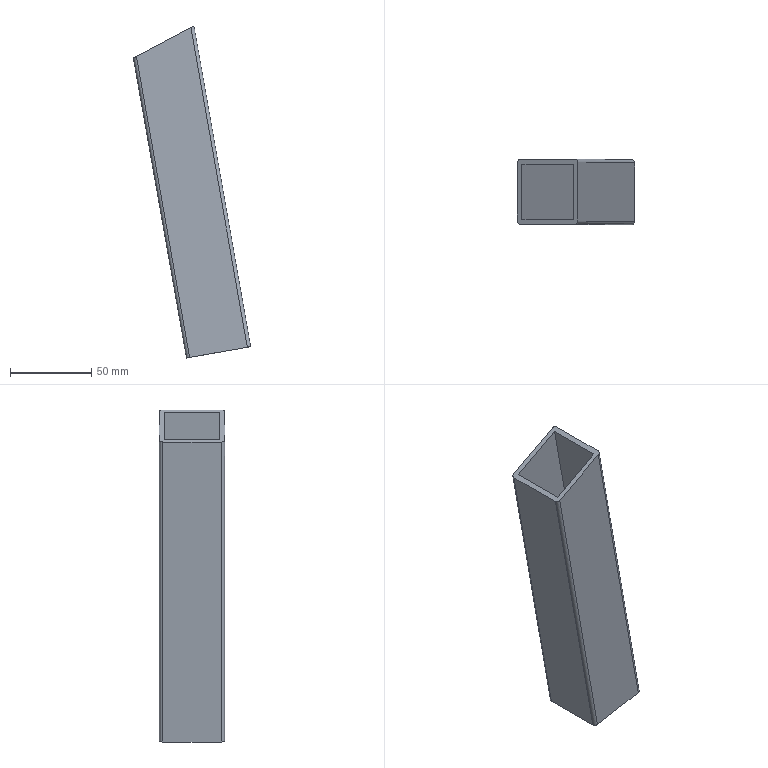Part | STEP file | diagonal bracket | 1 solid | 14 faces | box 71.941 x 40 x 203.909 mm | volume 85272 mm3 | plane 10 | cylinder 4 | commonest cylinder face diameters 4 x4
STEP:
#1=CARTESIAN_POINT('',(0.,0.,0.));
#2=DIRECTION('',(0.,0.,1.));
#3=DIRECTION('',(1.,0.,0.));
#4=AXIS2_PLACEMENT_3D('',#1,#2,#3);
#5=CARTESIAN_POINT('',(2102.233,153.75,-520.681));
#6=VERTEX_POINT('',#5);
#7=CARTESIAN_POINT('',(2068.752,153.75,-526.596));
#8=VERTEX_POINT('',#7);
#9=CARTESIAN_POINT('',(152.832,153.75,-865.079));
#10=DIRECTION('',(-0.9848,0.,-0.174));
#11=VECTOR('',#10,1.);
#12=LINE('',#9,#11);
#13=CARTESIAN_POINT('',(0.,153.75,0.));
#14=DIRECTION('',(0.,-1.,0.));
#15=DIRECTION('',(0.,0.,1.));
#16=AXIS2_PLACEMENT_3D('',#13,#14,#15);
#17=PLANE('',#16);
#18=CARTESIAN_POINT('',(-865.079,-152.832));
#19=DIRECTION('',(-0.174,0.9848));
#20=VECTOR('',#19,1.);
#21=LINE('',#18,#20);
#22=(GEOMETRIC_REPRESENTATION_CONTEXT(2)PARAMETRIC_REPRESENTATION_CONTEXT()REPRESENTATION_CONTEXT('',''));
#23=DEFINITIONAL_REPRESENTATION('',(#21),#22);
#24=PCURVE('',#17,#23);
#25=CARTESIAN_POINT('',(2105.187,190.75,-520.159));
#26=DIRECTION('',(-0.174,0.,0.9848));
#27=DIRECTION('',(-0.9848,0.,-0.174));
#28=AXIS2_PLACEMENT_3D('',#25,#26,#27);
#29=PLANE('',#28);
#30=CARTESIAN_POINT('',(1982.589,37.));
#31=DIRECTION('',(1.,0.));
#32=VECTOR('',#31,1.);
#33=LINE('',#30,#32);
#34=(GEOMETRIC_REPRESENTATION_CONTEXT(2)PARAMETRIC_REPRESENTATION_CONTEXT()REPRESENTATION_CONTEXT('',''));
#35=DEFINITIONAL_REPRESENTATION('',(#33),#34);
#36=PCURVE('',#29,#35);
#37=SURFACE_CURVE('',#12,(#24,#36),.PCURVE_S1.);
#38=EDGE_CURVE('',#6,#8,#37,.T.);
#39=ORIENTED_EDGE('',*,*,#38,.T.);
#40=CARTESIAN_POINT('',(2036.032,153.75,-341.393));
#41=VERTEX_POINT('',#40);
#42=CARTESIAN_POINT('',(2068.752,153.75,-526.596));
#43=DIRECTION('',(0.174,0.,-0.9848));
#44=VECTOR('',#43,1.);
#45=LINE('',#42,#44);
#46=CARTESIAN_POINT('',(-526.596,-2068.752));
#47=DIRECTION('',(-0.9848,-0.174));
#48=VECTOR('',#47,1.);
#49=LINE('',#46,#48);
#50=(GEOMETRIC_REPRESENTATION_CONTEXT(2)PARAMETRIC_REPRESENTATION_CONTEXT()REPRESENTATION_CONTEXT('',''));
#51=DEFINITIONAL_REPRESENTATION('',(#49),#50);
#52=PCURVE('',#17,#51);
#53=CARTESIAN_POINT('',(2068.752,190.75,-526.596));
#54=DIRECTION('',(0.9848,0.,0.174));
#55=DIRECTION('',(-0.174,0.,0.9848));
#56=AXIS2_PLACEMENT_3D('',#53,#54,#55);
#57=PLANE('',#56);
#58=CARTESIAN_POINT('',(0.,37.));
#59=DIRECTION('',(-1.,0.));
#60=VECTOR('',#59,1.);
#61=LINE('',#58,#60);
#62=(GEOMETRIC_REPRESENTATION_CONTEXT(2)PARAMETRIC_REPRESENTATION_CONTEXT()REPRESENTATION_CONTEXT('',''));
#63=DEFINITIONAL_REPRESENTATION('',(#61),#62);
#64=PCURVE('',#57,#63);
#65=SURFACE_CURVE('',#45,(#52,#64),.PCURVE_S1.);
#66=EDGE_CURVE('',#41,#8,#65,.T.);
#67=ORIENTED_EDGE('',*,*,#66,.F.);
#68=CARTESIAN_POINT('',(2067.606,153.75,-324.683));
#69=VERTEX_POINT('',#68);
#70=CARTESIAN_POINT('',(586.635,153.75,-1108.462));
#71=DIRECTION('',(0.8839,0.,0.4678));
#72=VECTOR('',#71,1.);
#73=LINE('',#70,#72);
#74=CARTESIAN_POINT('',(-1108.462,-586.635));
#75=DIRECTION('',(0.4678,-0.8839));
#76=VECTOR('',#75,1.);
#77=LINE('',#74,#76);
#78=(GEOMETRIC_REPRESENTATION_CONTEXT(2)PARAMETRIC_REPRESENTATION_CONTEXT()REPRESENTATION_CONTEXT('',''));
#79=DEFINITIONAL_REPRESENTATION('',(#77),#78);
#80=PCURVE('',#17,#79);
#81=CARTESIAN_POINT('',(2033.246,190.75,-342.868));
#82=DIRECTION('',(0.4678,0.,-0.8839));
#83=DIRECTION('',(0.8839,0.,0.4678));
#84=AXIS2_PLACEMENT_3D('',#81,#82,#83);
#85=PLANE('',#84);
#86=CARTESIAN_POINT('',(-1636.71,37.));
#87=DIRECTION('',(1.,0.));
#88=VECTOR('',#87,1.);
#89=LINE('',#86,#88);
#90=(GEOMETRIC_REPRESENTATION_CONTEXT(2)PARAMETRIC_REPRESENTATION_CONTEXT()REPRESENTATION_CONTEXT('',''));
#91=DEFINITIONAL_REPRESENTATION('',(#89),#90);
#92=PCURVE('',#85,#91);
#93=SURFACE_CURVE('',#73,(#80,#92),.PCURVE_S1.);
#94=EDGE_CURVE('',#41,#69,#93,.T.);
#95=ORIENTED_EDGE('',*,*,#94,.T.);
#96=CARTESIAN_POINT('',(2067.438,153.75,-323.73));
#97=DIRECTION('',(-0.174,0.,0.9848));
#98=VECTOR('',#97,1.);
#99=LINE('',#96,#98);
#100=CARTESIAN_POINT('',(-323.73,-2067.438));
#101=DIRECTION('',(0.9848,0.174));
#102=VECTOR('',#101,1.);
#103=LINE('',#100,#102);
#104=(GEOMETRIC_REPRESENTATION_CONTEXT(2)PARAMETRIC_REPRESENTATION_CONTEXT()REPRESENTATION_CONTEXT('',''));
#105=DEFINITIONAL_REPRESENTATION('',(#103),#104);
#106=PCURVE('',#17,#105);
#107=CARTESIAN_POINT('',(2067.438,190.75,-323.73));
#108=DIRECTION('',(-0.9848,0.,-0.174));
#109=DIRECTION('',(0.174,0.,-0.9848));
#110=AXIS2_PLACEMENT_3D('',#107,#108,#109);
#111=PLANE('',#110);
#112=CARTESIAN_POINT('',(0.,37.));
#113=DIRECTION('',(-1.,0.));
#114=VECTOR('',#113,1.);
#115=LINE('',#112,#114);
#116=(GEOMETRIC_REPRESENTATION_CONTEXT(2)PARAMETRIC_REPRESENTATION_CONTEXT()REPRESENTATION_CONTEXT('',''));
#117=DEFINITIONAL_REPRESENTATION('',(#115),#116);
#118=PCURVE('',#111,#117);
#119=SURFACE_CURVE('',#99,(#106,#118),.PCURVE_S1.);
#120=EDGE_CURVE('',#6,#69,#119,.T.);
#121=ORIENTED_EDGE('',*,*,#120,.F.);
#122=EDGE_LOOP('',(#39,#67,#95,#121));
#123=FACE_BOUND('',#122,.T.);
#124=ADVANCED_FACE('',(#123),#17,.F.);
#125=CARTESIAN_POINT('',(2036.032,187.75,-341.393));
#126=VERTEX_POINT('',#125);
#127=CARTESIAN_POINT('',(2067.606,187.75,-324.683));
#128=VERTEX_POINT('',#127);
#129=CARTESIAN_POINT('',(586.635,187.75,-1108.462));
#130=DIRECTION('',(0.8839,0.,0.4678));
#131=VECTOR('',#130,1.);
#132=LINE('',#129,#131);
#133=CARTESIAN_POINT('',(0.,187.75,0.));
#134=DIRECTION('',(0.,-1.,0.));
#135=DIRECTION('',(0.,0.,1.));
#136=AXIS2_PLACEMENT_3D('',#133,#134,#135);
#137=PLANE('',#136);
#138=CARTESIAN_POINT('',(-1108.462,-586.635));
#139=DIRECTION('',(0.4678,-0.8839));
#140=VECTOR('',#139,1.);
#141=LINE('',#138,#140);
#142=(GEOMETRIC_REPRESENTATION_CONTEXT(2)PARAMETRIC_REPRESENTATION_CONTEXT()REPRESENTATION_CONTEXT('',''));
#143=DEFINITIONAL_REPRESENTATION('',(#141),#142);
#144=PCURVE('',#137,#143);
#145=CARTESIAN_POINT('',(-1636.71,3.));
#146=DIRECTION('',(1.,0.));
#147=VECTOR('',#146,1.);
#148=LINE('',#145,#147);
#149=(GEOMETRIC_REPRESENTATION_CONTEXT(2)PARAMETRIC_REPRESENTATION_CONTEXT()REPRESENTATION_CONTEXT('',''));
#150=DEFINITIONAL_REPRESENTATION('',(#148),#149);
#151=PCURVE('',#85,#150);
#152=SURFACE_CURVE('',#132,(#144,#151),.PCURVE_S1.);
#153=EDGE_CURVE('',#126,#128,#152,.T.);
#154=ORIENTED_EDGE('',*,*,#153,.F.);
#155=CARTESIAN_POINT('',(2068.752,187.75,-526.596));
#156=VERTEX_POINT('',#155);
#157=CARTESIAN_POINT('',(2068.752,187.75,-526.596));
#158=DIRECTION('',(0.174,0.,-0.9848));
#159=VECTOR('',#158,1.);
#160=LINE('',#157,#159);
#161=CARTESIAN_POINT('',(-526.596,-2068.752));
#162=DIRECTION('',(-0.9848,-0.174));
#163=VECTOR('',#162,1.);
#164=LINE('',#161,#163);
#165=(GEOMETRIC_REPRESENTATION_CONTEXT(2)PARAMETRIC_REPRESENTATION_CONTEXT()REPRESENTATION_CONTEXT('',''));
#166=DEFINITIONAL_REPRESENTATION('',(#164),#165);
#167=PCURVE('',#137,#166);
#168=CARTESIAN_POINT('',(0.,3.));
#169=DIRECTION('',(-1.,0.));
#170=VECTOR('',#169,1.);
#171=LINE('',#168,#170);
#172=(GEOMETRIC_REPRESENTATION_CONTEXT(2)PARAMETRIC_REPRESENTATION_CONTEXT()REPRESENTATION_CONTEXT('',''));
#173=DEFINITIONAL_REPRESENTATION('',(#171),#172);
#174=PCURVE('',#57,#173);
#175=SURFACE_CURVE('',#160,(#167,#174),.PCURVE_S1.);
#176=EDGE_CURVE('',#126,#156,#175,.T.);
#177=ORIENTED_EDGE('',*,*,#176,.T.);
#178=CARTESIAN_POINT('',(2102.233,187.75,-520.681));
#179=VERTEX_POINT('',#178);
#180=CARTESIAN_POINT('',(152.832,187.75,-865.079));
#181=DIRECTION('',(-0.9848,0.,-0.174));
#182=VECTOR('',#181,1.);
#183=LINE('',#180,#182);
#184=CARTESIAN_POINT('',(-865.079,-152.832));
#185=DIRECTION('',(-0.174,0.9848));
#186=VECTOR('',#185,1.);
#187=LINE('',#184,#186);
#188=(GEOMETRIC_REPRESENTATION_CONTEXT(2)PARAMETRIC_REPRESENTATION_CONTEXT()REPRESENTATION_CONTEXT('',''));
#189=DEFINITIONAL_REPRESENTATION('',(#187),#188);
#190=PCURVE('',#137,#189);
#191=CARTESIAN_POINT('',(1982.589,3.));
#192=DIRECTION('',(1.,0.));
#193=VECTOR('',#192,1.);
#194=LINE('',#191,#193);
#195=(GEOMETRIC_REPRESENTATION_CONTEXT(2)PARAMETRIC_REPRESENTATION_CONTEXT()REPRESENTATION_CONTEXT('',''));
#196=DEFINITIONAL_REPRESENTATION('',(#194),#195);
#197=PCURVE('',#29,#196);
#198=SURFACE_CURVE('',#183,(#190,#197),.PCURVE_S1.);
#199=EDGE_CURVE('',#179,#156,#198,.T.);
#200=ORIENTED_EDGE('',*,*,#199,.F.);
#201=CARTESIAN_POINT('',(2067.438,187.75,-323.73));
#202=DIRECTION('',(-0.174,0.,0.9848));
#203=VECTOR('',#202,1.);
#204=LINE('',#201,#203);
#205=CARTESIAN_POINT('',(-323.73,-2067.438));
#206=DIRECTION('',(0.9848,0.174));
#207=VECTOR('',#206,1.);
#208=LINE('',#205,#207);
#209=(GEOMETRIC_REPRESENTATION_CONTEXT(2)PARAMETRIC_REPRESENTATION_CONTEXT()REPRESENTATION_CONTEXT('',''));
#210=DEFINITIONAL_REPRESENTATION('',(#208),#209);
#211=PCURVE('',#137,#210);
#212=CARTESIAN_POINT('',(0.,3.));
#213=DIRECTION('',(-1.,0.));
#214=VECTOR('',#213,1.);
#215=LINE('',#212,#214);
#216=(GEOMETRIC_REPRESENTATION_CONTEXT(2)PARAMETRIC_REPRESENTATION_CONTEXT()REPRESENTATION_CONTEXT('',''));
#217=DEFINITIONAL_REPRESENTATION('',(#215),#216);
#218=PCURVE('',#111,#217);
#219=SURFACE_CURVE('',#204,(#211,#218),.PCURVE_S1.);
#220=EDGE_CURVE('',#179,#128,#219,.T.);
#221=ORIENTED_EDGE('',*,*,#220,.T.);
#222=EDGE_LOOP('',(#154,#177,#200,#221));
#223=FACE_BOUND('',#222,.T.);
#224=ADVANCED_FACE('',(#223),#137,.T.);
#225=CARTESIAN_POINT('',(2067.606,190.75,-324.683));
#226=DIRECTION('',(0.,-1.,0.));
#227=VECTOR('',#226,1.);
#228=LINE('',#225,#227);
#229=CARTESIAN_POINT('',(0.9673,0.));
#230=DIRECTION('',(0.,1.));
#231=VECTOR('',#230,1.);
#232=LINE('',#229,#231);
#233=(GEOMETRIC_REPRESENTATION_CONTEXT(2)PARAMETRIC_REPRESENTATION_CONTEXT()REPRESENTATION_CONTEXT('',''));
#234=DEFINITIONAL_REPRESENTATION('',(#232),#233);
#235=PCURVE('',#111,#234);
#236=CARTESIAN_POINT('',(38.876,0.));
#237=DIRECTION('',(0.,1.));
#238=VECTOR('',#237,1.);
#239=LINE('',#236,#238);
#240=(GEOMETRIC_REPRESENTATION_CONTEXT(2)PARAMETRIC_REPRESENTATION_CONTEXT()REPRESENTATION_CONTEXT('',''));
#241=DEFINITIONAL_REPRESENTATION('',(#239),#240);
#242=PCURVE('',#85,#241);
#243=SURFACE_CURVE('',#228,(#235,#242),.PCURVE_S1.);
#244=EDGE_CURVE('',#128,#69,#243,.T.);
#245=ORIENTED_EDGE('',*,*,#244,.F.);
#246=ORIENTED_EDGE('',*,*,#220,.F.);
#247=CARTESIAN_POINT('',(2102.233,190.75,-520.681));
#248=DIRECTION('',(0.,-1.,0.));
#249=VECTOR('',#248,1.);
#250=LINE('',#247,#249);
#251=CARTESIAN_POINT('',(200.,0.));
#252=DIRECTION('',(0.,1.));
#253=VECTOR('',#252,1.);
#254=LINE('',#251,#253);
#255=(GEOMETRIC_REPRESENTATION_CONTEXT(2)PARAMETRIC_REPRESENTATION_CONTEXT()REPRESENTATION_CONTEXT('',''));
#256=DEFINITIONAL_REPRESENTATION('',(#254),#255);
#257=PCURVE('',#111,#256);
#258=CARTESIAN_POINT('',(3.,0.));
#259=DIRECTION('',(0.,1.));
#260=VECTOR('',#259,1.);
#261=LINE('',#258,#260);
#262=(GEOMETRIC_REPRESENTATION_CONTEXT(2)PARAMETRIC_REPRESENTATION_CONTEXT()REPRESENTATION_CONTEXT('',''));
#263=DEFINITIONAL_REPRESENTATION('',(#261),#262);
#264=PCURVE('',#29,#263);
#265=SURFACE_CURVE('',#250,(#257,#264),.PCURVE_S1.);
#266=EDGE_CURVE('',#179,#6,#265,.T.);
#267=ORIENTED_EDGE('',*,*,#266,.T.);
#268=ORIENTED_EDGE('',*,*,#120,.T.);
#269=EDGE_LOOP('',(#245,#246,#267,#268));
#270=FACE_BOUND('',#269,.T.);
#271=ADVANCED_FACE('',(#270),#111,.T.);
#272=CARTESIAN_POINT('',(2068.752,190.75,-526.596));
#273=DIRECTION('',(0.,-1.,0.));
#274=VECTOR('',#273,1.);
#275=LINE('',#272,#274);
#276=CARTESIAN_POINT('',(0.,0.));
#277=DIRECTION('',(0.,1.));
#278=VECTOR('',#277,1.);
#279=LINE('',#276,#278);
#280=(GEOMETRIC_REPRESENTATION_CONTEXT(2)PARAMETRIC_REPRESENTATION_CONTEXT()REPRESENTATION_CONTEXT('',''));
#281=DEFINITIONAL_REPRESENTATION('',(#279),#280);
#282=PCURVE('',#57,#281);
#283=CARTESIAN_POINT('',(37.,0.));
#284=DIRECTION('',(0.,1.));
#285=VECTOR('',#284,1.);
#286=LINE('',#283,#285);
#287=(GEOMETRIC_REPRESENTATION_CONTEXT(2)PARAMETRIC_REPRESENTATION_CONTEXT()REPRESENTATION_CONTEXT('',''));
#288=DEFINITIONAL_REPRESENTATION('',(#286),#287);
#289=PCURVE('',#29,#288);
#290=SURFACE_CURVE('',#275,(#282,#289),.PCURVE_S1.);
#291=EDGE_CURVE('',#156,#8,#290,.T.);
#292=ORIENTED_EDGE('',*,*,#291,.F.);
#293=ORIENTED_EDGE('',*,*,#176,.F.);
#294=CARTESIAN_POINT('',(2036.032,190.75,-341.393));
#295=DIRECTION('',(0.,-1.,0.));
#296=VECTOR('',#295,1.);
#297=LINE('',#294,#296);
#298=CARTESIAN_POINT('',(188.071,0.));
#299=DIRECTION('',(0.,1.));
#300=VECTOR('',#299,1.);
#301=LINE('',#298,#300);
#302=(GEOMETRIC_REPRESENTATION_CONTEXT(2)PARAMETRIC_REPRESENTATION_CONTEXT()REPRESENTATION_CONTEXT('',''));
#303=DEFINITIONAL_REPRESENTATION('',(#301),#302);
#304=PCURVE('',#57,#303);
#305=CARTESIAN_POINT('',(3.152,0.));
#306=DIRECTION('',(0.,1.));
#307=VECTOR('',#306,1.);
#308=LINE('',#305,#307);
#309=(GEOMETRIC_REPRESENTATION_CONTEXT(2)PARAMETRIC_REPRESENTATION_CONTEXT()REPRESENTATION_CONTEXT('',''));
#310=DEFINITIONAL_REPRESENTATION('',(#308),#309);
#311=PCURVE('',#85,#310);
#312=SURFACE_CURVE('',#297,(#304,#311),.PCURVE_S1.);
#313=EDGE_CURVE('',#126,#41,#312,.T.);
#314=ORIENTED_EDGE('',*,*,#313,.T.);
#315=ORIENTED_EDGE('',*,*,#66,.T.);
#316=EDGE_LOOP('',(#292,#293,#314,#315));
#317=FACE_BOUND('',#316,.T.);
#318=ADVANCED_FACE('',(#317),#57,.T.);
#319=CARTESIAN_POINT('',(2065.797,188.75,-527.118));
#320=VERTEX_POINT('',#319);
#321=CARTESIAN_POINT('',(2067.767,190.75,-526.77));
#322=VERTEX_POINT('',#321);
#323=CARTESIAN_POINT('',(2067.767,188.75,-526.77));
#324=DIRECTION('',(0.174,0.,-0.9848));
#325=DIRECTION('',(0.9848,0.,0.174));
#326=AXIS2_PLACEMENT_3D('',#323,#324,#325);
#327=CIRCLE('',#326,2.);
#328=CARTESIAN_POINT('',(1914.935,188.75,338.309));
#329=DIRECTION('',(-0.174,0.,0.9848));
#330=DIRECTION('',(-0.9848,0.,-0.174));
#331=AXIS2_PLACEMENT_3D('',#328,#329,#330);
#332=CYLINDRICAL_SURFACE('',#331,2.);
#333=CARTESIAN_POINT('',(9.425,-878.475));
#334=DIRECTION('',(-1.,0.));
#335=VECTOR('',#334,1.);
#336=LINE('',#333,#335);
#337=(GEOMETRIC_REPRESENTATION_CONTEXT(2)PARAMETRIC_REPRESENTATION_CONTEXT()REPRESENTATION_CONTEXT('',''));
#338=DEFINITIONAL_REPRESENTATION('',(#336),#337);
#339=PCURVE('',#332,#338);
#340=CARTESIAN_POINT('',(36.,2.));
#341=CARTESIAN_POINT('',(36.,5.464));
#342=CARTESIAN_POINT('',(39.,3.732));
#343=CARTESIAN_POINT('',(42.,2.));
#344=CARTESIAN_POINT('',(39.,0.2679));
#345=CARTESIAN_POINT('',(36.,-1.464));
#346=CARTESIAN_POINT('',(36.,2.));
#347=(BOUNDED_CURVE()B_SPLINE_CURVE(2,(#340,#341,#342,#343,#344,#345,#346),.UNSPECIFIED.,.T.,.F.)B_SPLINE_CURVE_WITH_KNOTS((1,2,2,2,2,1),(-2.094,0.,2.094,4.189,6.283,8.378),.UNSPECIFIED.)CURVE()GEOMETRIC_REPRESENTATION_ITEM()RATIONAL_B_SPLINE_CURVE((1.,0.5,1.,0.5,1.,0.5,1.))REPRESENTATION_ITEM(''));
#348=(GEOMETRIC_REPRESENTATION_CONTEXT(2)PARAMETRIC_REPRESENTATION_CONTEXT()REPRESENTATION_CONTEXT('',''));
#349=DEFINITIONAL_REPRESENTATION('',(#347),#348);
#350=PCURVE('',#29,#349);
#351=SURFACE_CURVE('',#327,(#339,#350),.PCURVE_S1.);
#352=EDGE_CURVE('',#320,#322,#351,.T.);
#353=ORIENTED_EDGE('',*,*,#352,.F.);
#354=CARTESIAN_POINT('',(2033.246,188.75,-342.868));
#355=VERTEX_POINT('',#354);
#356=CARTESIAN_POINT('',(2065.797,188.75,-527.118));
#357=DIRECTION('',(0.174,0.,-0.9848));
#358=VECTOR('',#357,1.);
#359=LINE('',#356,#358);
#360=CARTESIAN_POINT('',(6.283,-878.475));
#361=DIRECTION('',(0.,-1.));
#362=VECTOR('',#361,1.);
#363=LINE('',#360,#362);
#364=(GEOMETRIC_REPRESENTATION_CONTEXT(2)PARAMETRIC_REPRESENTATION_CONTEXT()REPRESENTATION_CONTEXT('',''));
#365=DEFINITIONAL_REPRESENTATION('',(#363),#364);
#366=PCURVE('',#332,#365);
#367=CARTESIAN_POINT('',(2065.797,190.75,-527.118));
#368=DIRECTION('',(0.9848,0.,0.174));
#369=DIRECTION('',(-0.174,0.,0.9848));
#370=AXIS2_PLACEMENT_3D('',#367,#368,#369);
#371=PLANE('',#370);
#372=CARTESIAN_POINT('',(0.,2.));
#373=DIRECTION('',(-1.,0.));
#374=VECTOR('',#373,1.);
#375=LINE('',#372,#374);
#376=(GEOMETRIC_REPRESENTATION_CONTEXT(2)PARAMETRIC_REPRESENTATION_CONTEXT()REPRESENTATION_CONTEXT('',''));
#377=DEFINITIONAL_REPRESENTATION('',(#375),#376);
#378=PCURVE('',#371,#377);
#379=SURFACE_CURVE('',#359,(#366,#378),.PCURVE_S1.);
#380=EDGE_CURVE('',#355,#320,#379,.T.);
#381=ORIENTED_EDGE('',*,*,#380,.F.);
#382=CARTESIAN_POINT('',(2035.103,190.75,-341.885));
#383=VERTEX_POINT('',#382);
#384=CARTESIAN_POINT('',(2035.103,188.75,-341.885));
#385=DIRECTION('',(-0.4678,0.,0.8839));
#386=DIRECTION('',(0.8839,0.,0.4678));
#387=AXIS2_PLACEMENT_3D('',#384,#385,#386);
#388=ELLIPSE('',#387,2.101,2.);
#389=CARTESIAN_POINT('',(4.712,-690.727));
#390=CARTESIAN_POINT('',(4.736,-690.742));
#391=CARTESIAN_POINT('',(4.784,-690.773));
#392=CARTESIAN_POINT('',(4.855,-690.819));
#393=CARTESIAN_POINT('',(4.927,-690.864));
#394=CARTESIAN_POINT('',(4.998,-690.909));
#395=CARTESIAN_POINT('',(5.069,-690.953));
#396=CARTESIAN_POINT('',(5.141,-690.995));
#397=CARTESIAN_POINT('',(5.212,-691.036));
#398=CARTESIAN_POINT('',(5.284,-691.076));
#399=CARTESIAN_POINT('',(5.355,-691.114));
#400=CARTESIAN_POINT('',(5.426,-691.15));
#401=CARTESIAN_POINT('',(5.498,-691.183));
#402=CARTESIAN_POINT('',(5.569,-691.215));
#403=CARTESIAN_POINT('',(5.641,-691.244));
#404=CARTESIAN_POINT('',(5.712,-691.27));
#405=CARTESIAN_POINT('',(5.783,-691.294));
#406=CARTESIAN_POINT('',(5.855,-691.314));
#407=CARTESIAN_POINT('',(5.926,-691.332));
#408=CARTESIAN_POINT('',(5.998,-691.346));
#409=CARTESIAN_POINT('',(6.069,-691.358));
#410=CARTESIAN_POINT('',(6.14,-691.366));
#411=CARTESIAN_POINT('',(6.212,-691.371));
#412=CARTESIAN_POINT('',(6.259,-691.372));
#413=CARTESIAN_POINT('',(6.283,-691.372));
#414=B_SPLINE_CURVE_WITH_KNOTS('',3,(#389,#390,#391,#392,#393,#394,#395,#396,#397,#398,#399,#400,#401,#402,#403,#404,#405,#406,#407,#408,#409,#410,#411,#412,#413),.UNSPECIFIED.,.F.,.F.,(4,1,1,1,1,1,1,1,1,1,1,1,1,1,1,1,1,1,1,1,1,1,4),(1.571,1.642,1.714,1.785,1.856,1.928,1.999,2.071,2.142,2.213,2.285,2.356,2.428,2.499,2.57,2.642,2.713,2.785,2.856,2.927,2.999,3.07,3.142),.QUASI_UNIFORM_KNOTS.);
#415=(GEOMETRIC_REPRESENTATION_CONTEXT(2)PARAMETRIC_REPRESENTATION_CONTEXT()REPRESENTATION_CONTEXT('',''));
#416=DEFINITIONAL_REPRESENTATION('',(#414),#415);
#417=PCURVE('',#332,#416);
#418=CARTESIAN_POINT('',(4.203,2.));
#419=CARTESIAN_POINT('',(4.203,-1.464));
#420=CARTESIAN_POINT('',(1.051,0.2679));
#421=CARTESIAN_POINT('',(-2.101,2.));
#422=CARTESIAN_POINT('',(1.051,3.732));
#423=CARTESIAN_POINT('',(4.203,5.464));
#424=CARTESIAN_POINT('',(4.203,2.));
#425=(BOUNDED_CURVE()B_SPLINE_CURVE(2,(#418,#419,#420,#421,#422,#423,#424),.UNSPECIFIED.,.T.,.F.)B_SPLINE_CURVE_WITH_KNOTS((1,2,2,2,2,1),(-2.094,0.,2.094,4.189,6.283,8.378),.UNSPECIFIED.)CURVE()GEOMETRIC_REPRESENTATION_ITEM()RATIONAL_B_SPLINE_CURVE((1.,0.5,1.,0.5,1.,0.5,1.))REPRESENTATION_ITEM(''));
#426=(GEOMETRIC_REPRESENTATION_CONTEXT(2)PARAMETRIC_REPRESENTATION_CONTEXT()REPRESENTATION_CONTEXT('',''));
#427=DEFINITIONAL_REPRESENTATION('',(#425),#426);
#428=PCURVE('',#85,#427);
#429=SURFACE_CURVE('',#388,(#417,#428),.PCURVE_S1.);
#430=EDGE_CURVE('',#383,#355,#429,.T.);
#431=ORIENTED_EDGE('',*,*,#430,.F.);
#432=CARTESIAN_POINT('',(1914.935,190.75,338.309));
#433=DIRECTION('',(-0.174,0.,0.9848));
#434=VECTOR('',#433,1.);
#435=LINE('',#432,#434);
#436=CARTESIAN_POINT('',(4.712,0.));
#437=DIRECTION('',(0.,1.));
#438=VECTOR('',#437,1.);
#439=LINE('',#436,#438);
#440=(GEOMETRIC_REPRESENTATION_CONTEXT(2)PARAMETRIC_REPRESENTATION_CONTEXT()REPRESENTATION_CONTEXT('',''));
#441=DEFINITIONAL_REPRESENTATION('',(#439),#440);
#442=PCURVE('',#332,#441);
#443=CARTESIAN_POINT('',(0.,190.75,0.));
#444=DIRECTION('',(0.,-1.,0.));
#445=DIRECTION('',(0.,0.,1.));
#446=AXIS2_PLACEMENT_3D('',#443,#444,#445);
#447=PLANE('',#446);
#448=CARTESIAN_POINT('',(338.309,-1914.935));
#449=DIRECTION('',(0.9848,0.174));
#450=VECTOR('',#449,1.);
#451=LINE('',#448,#450);
#452=(GEOMETRIC_REPRESENTATION_CONTEXT(2)PARAMETRIC_REPRESENTATION_CONTEXT()REPRESENTATION_CONTEXT('',''));
#453=DEFINITIONAL_REPRESENTATION('',(#451),#452);
#454=PCURVE('',#447,#453);
#455=SURFACE_CURVE('',#435,(#442,#454),.PCURVE_S1.);
#456=EDGE_CURVE('',#322,#383,#455,.T.);
#457=ORIENTED_EDGE('',*,*,#456,.F.);
#458=EDGE_LOOP('',(#353,#381,#431,#457));
#459=FACE_BOUND('',#458,.T.);
#460=ADVANCED_FACE('',(#459),#332,.T.);
#461=CARTESIAN_POINT('',(2070.392,188.75,-323.209));
#462=VERTEX_POINT('',#461);
#463=CARTESIAN_POINT('',(2068.535,190.75,-324.192));
#464=VERTEX_POINT('',#463);
#465=CARTESIAN_POINT('',(2068.535,188.75,-324.192));
#466=DIRECTION('',(-0.4678,0.,0.8839));
#467=DIRECTION('',(-0.8839,0.,-0.4678));
#468=AXIS2_PLACEMENT_3D('',#465,#466,#467);
#469=ELLIPSE('',#468,2.101,2.);
#470=CARTESIAN_POINT('',(1950.386,188.75,344.572));
#471=DIRECTION('',(0.174,0.,-0.9848));
#472=DIRECTION('',(0.9848,0.,0.174));
#473=AXIS2_PLACEMENT_3D('',#470,#471,#472);
#474=CYLINDRICAL_SURFACE('',#473,2.);
#475=CARTESIAN_POINT('',(6.283,678.475));
#476=CARTESIAN_POINT('',(6.259,678.475));
#477=CARTESIAN_POINT('',(6.212,678.476));
#478=CARTESIAN_POINT('',(6.14,678.481));
#479=CARTESIAN_POINT('',(6.069,678.489));
#480=CARTESIAN_POINT('',(5.998,678.501));
#481=CARTESIAN_POINT('',(5.926,678.515));
#482=CARTESIAN_POINT('',(5.855,678.533));
#483=CARTESIAN_POINT('',(5.783,678.554));
#484=CARTESIAN_POINT('',(5.712,678.577));
#485=CARTESIAN_POINT('',(5.641,678.603));
#486=CARTESIAN_POINT('',(5.569,678.632));
#487=CARTESIAN_POINT('',(5.498,678.664));
#488=CARTESIAN_POINT('',(5.426,678.697));
#489=CARTESIAN_POINT('',(5.355,678.733));
#490=CARTESIAN_POINT('',(5.284,678.771));
#491=CARTESIAN_POINT('',(5.212,678.811));
#492=CARTESIAN_POINT('',(5.141,678.852));
#493=CARTESIAN_POINT('',(5.069,678.895));
#494=CARTESIAN_POINT('',(4.998,678.938));
#495=CARTESIAN_POINT('',(4.927,678.983));
#496=CARTESIAN_POINT('',(4.855,679.028));
#497=CARTESIAN_POINT('',(4.784,679.074));
#498=CARTESIAN_POINT('',(4.736,679.105));
#499=CARTESIAN_POINT('',(4.712,679.12));
#500=B_SPLINE_CURVE_WITH_KNOTS('',3,(#475,#476,#477,#478,#479,#480,#481,#482,#483,#484,#485,#486,#487,#488,#489,#490,#491,#492,#493,#494,#495,#496,#497,#498,#499),.UNSPECIFIED.,.F.,.F.,(4,1,1,1,1,1,1,1,1,1,1,1,1,1,1,1,1,1,1,1,1,1,4),(3.142,3.213,3.284,3.356,3.427,3.499,3.57,3.641,3.713,3.784,3.856,3.927,3.998,4.07,4.141,4.213,4.284,4.355,4.427,4.498,4.57,4.641,4.712),.QUASI_UNIFORM_KNOTS.);
#501=(GEOMETRIC_REPRESENTATION_CONTEXT(2)PARAMETRIC_REPRESENTATION_CONTEXT()REPRESENTATION_CONTEXT('',''));
#502=DEFINITIONAL_REPRESENTATION('',(#500),#501);
#503=PCURVE('',#474,#502);
#504=CARTESIAN_POINT('',(37.825,2.));
#505=CARTESIAN_POINT('',(37.825,5.464));
#506=CARTESIAN_POINT('',(40.977,3.732));
#507=CARTESIAN_POINT('',(44.129,2.));
#508=CARTESIAN_POINT('',(40.977,0.2679));
#509=CARTESIAN_POINT('',(37.825,-1.464));
#510=CARTESIAN_POINT('',(37.825,2.));
#511=(BOUNDED_CURVE()B_SPLINE_CURVE(2,(#504,#505,#506,#507,#508,#509,#510),.UNSPECIFIED.,.T.,.F.)B_SPLINE_CURVE_WITH_KNOTS((1,2,2,2,2,1),(-2.094,0.,2.094,4.189,6.283,8.378),.UNSPECIFIED.)CURVE()GEOMETRIC_REPRESENTATION_ITEM()RATIONAL_B_SPLINE_CURVE((1.,0.5,1.,0.5,1.,0.5,1.))REPRESENTATION_ITEM(''));
#512=(GEOMETRIC_REPRESENTATION_CONTEXT(2)PARAMETRIC_REPRESENTATION_CONTEXT()REPRESENTATION_CONTEXT('',''));
#513=DEFINITIONAL_REPRESENTATION('',(#511),#512);
#514=PCURVE('',#85,#513);
#515=SURFACE_CURVE('',#469,(#503,#514),.PCURVE_S1.);
#516=EDGE_CURVE('',#462,#464,#515,.T.);
#517=ORIENTED_EDGE('',*,*,#516,.F.);
#518=CARTESIAN_POINT('',(2105.187,188.75,-520.159));
#519=VERTEX_POINT('',#518);
#520=CARTESIAN_POINT('',(2070.392,188.75,-323.209));
#521=DIRECTION('',(-0.174,0.,0.9848));
#522=VECTOR('',#521,1.);
#523=LINE('',#520,#522);
#524=CARTESIAN_POINT('',(6.283,678.475));
#525=DIRECTION('',(0.,-1.));
#526=VECTOR('',#525,1.);
#527=LINE('',#524,#526);
#528=(GEOMETRIC_REPRESENTATION_CONTEXT(2)PARAMETRIC_REPRESENTATION_CONTEXT()REPRESENTATION_CONTEXT('',''));
#529=DEFINITIONAL_REPRESENTATION('',(#527),#528);
#530=PCURVE('',#474,#529);
#531=CARTESIAN_POINT('',(2070.392,190.75,-323.209));
#532=DIRECTION('',(-0.9848,0.,-0.174));
#533=DIRECTION('',(0.174,0.,-0.9848));
#534=AXIS2_PLACEMENT_3D('',#531,#532,#533);
#535=PLANE('',#534);
#536=CARTESIAN_POINT('',(0.,2.));
#537=DIRECTION('',(-1.,0.));
#538=VECTOR('',#537,1.);
#539=LINE('',#536,#538);
#540=(GEOMETRIC_REPRESENTATION_CONTEXT(2)PARAMETRIC_REPRESENTATION_CONTEXT()REPRESENTATION_CONTEXT('',''));
#541=DEFINITIONAL_REPRESENTATION('',(#539),#540);
#542=PCURVE('',#535,#541);
#543=SURFACE_CURVE('',#523,(#530,#542),.PCURVE_S1.);
#544=EDGE_CURVE('',#519,#462,#543,.T.);
#545=ORIENTED_EDGE('',*,*,#544,.F.);
#546=CARTESIAN_POINT('',(2103.218,190.75,-520.507));
#547=VERTEX_POINT('',#546);
#548=CARTESIAN_POINT('',(2103.218,188.75,-520.507));
#549=DIRECTION('',(0.174,0.,-0.9848));
#550=DIRECTION('',(0.9848,0.,0.174));
#551=AXIS2_PLACEMENT_3D('',#548,#549,#550);
#552=CIRCLE('',#551,2.);
#553=CARTESIAN_POINT('',(0.,878.475));
#554=DIRECTION('',(1.,0.));
#555=VECTOR('',#554,1.);
#556=LINE('',#553,#555);
#557=(GEOMETRIC_REPRESENTATION_CONTEXT(2)PARAMETRIC_REPRESENTATION_CONTEXT()REPRESENTATION_CONTEXT('',''));
#558=DEFINITIONAL_REPRESENTATION('',(#556),#557);
#559=PCURVE('',#474,#558);
#560=CARTESIAN_POINT('',(0.,2.));
#561=CARTESIAN_POINT('',(0.,5.464));
#562=CARTESIAN_POINT('',(3.,3.732));
#563=CARTESIAN_POINT('',(6.,2.));
#564=CARTESIAN_POINT('',(3.,0.2679));
#565=CARTESIAN_POINT('',(0.,-1.464));
#566=CARTESIAN_POINT('',(0.,2.));
#567=(BOUNDED_CURVE()B_SPLINE_CURVE(2,(#560,#561,#562,#563,#564,#565,#566),.UNSPECIFIED.,.T.,.F.)B_SPLINE_CURVE_WITH_KNOTS((1,2,2,2,2,1),(-2.094,0.,2.094,4.189,6.283,8.378),.UNSPECIFIED.)CURVE()GEOMETRIC_REPRESENTATION_ITEM()RATIONAL_B_SPLINE_CURVE((1.,0.5,1.,0.5,1.,0.5,1.))REPRESENTATION_ITEM(''));
#568=(GEOMETRIC_REPRESENTATION_CONTEXT(2)PARAMETRIC_REPRESENTATION_CONTEXT()REPRESENTATION_CONTEXT('',''));
#569=DEFINITIONAL_REPRESENTATION('',(#567),#568);
#570=PCURVE('',#29,#569);
#571=SURFACE_CURVE('',#552,(#559,#570),.PCURVE_S1.);
#572=EDGE_CURVE('',#547,#519,#571,.T.);
#573=ORIENTED_EDGE('',*,*,#572,.F.);
#574=CARTESIAN_POINT('',(1950.386,190.75,344.572));
#575=DIRECTION('',(0.174,0.,-0.9848));
#576=VECTOR('',#575,1.);
#577=LINE('',#574,#576);
#578=CARTESIAN_POINT('',(4.712,0.));
#579=DIRECTION('',(0.,1.));
#580=VECTOR('',#579,1.);
#581=LINE('',#578,#580);
#582=(GEOMETRIC_REPRESENTATION_CONTEXT(2)PARAMETRIC_REPRESENTATION_CONTEXT()REPRESENTATION_CONTEXT('',''));
#583=DEFINITIONAL_REPRESENTATION('',(#581),#582);
#584=PCURVE('',#474,#583);
#585=CARTESIAN_POINT('',(344.572,-1950.386));
#586=DIRECTION('',(-0.9848,-0.174));
#587=VECTOR('',#586,1.);
#588=LINE('',#585,#587);
#589=(GEOMETRIC_REPRESENTATION_CONTEXT(2)PARAMETRIC_REPRESENTATION_CONTEXT()REPRESENTATION_CONTEXT('',''));
#590=DEFINITIONAL_REPRESENTATION('',(#588),#589);
#591=PCURVE('',#447,#590);
#592=SURFACE_CURVE('',#577,(#584,#591),.PCURVE_S1.);
#593=EDGE_CURVE('',#464,#547,#592,.T.);
#594=ORIENTED_EDGE('',*,*,#593,.F.);
#595=EDGE_LOOP('',(#517,#545,#573,#594));
#596=FACE_BOUND('',#595,.T.);
#597=ADVANCED_FACE('',(#596),#474,.T.);
#598=CARTESIAN_POINT('',(2067.767,150.75,-526.77));
#599=VERTEX_POINT('',#598);
#600=CARTESIAN_POINT('',(2065.797,152.75,-527.118));
#601=VERTEX_POINT('',#600);
#602=CARTESIAN_POINT('',(2067.767,152.75,-526.77));
#603=DIRECTION('',(0.174,0.,-0.9848));
#604=DIRECTION('',(0.9848,0.,0.174));
#605=AXIS2_PLACEMENT_3D('',#602,#603,#604);
#606=CIRCLE('',#605,2.);
#607=CARTESIAN_POINT('',(2067.767,152.75,-526.77));
#608=DIRECTION('',(0.174,0.,-0.9848));
#609=DIRECTION('',(0.9848,0.,0.174));
#610=AXIS2_PLACEMENT_3D('',#607,#608,#609);
#611=CYLINDRICAL_SURFACE('',#610,2.);
#612=CARTESIAN_POINT('',(0.,0.));
#613=DIRECTION('',(1.,0.));
#614=VECTOR('',#613,1.);
#615=LINE('',#612,#614);
#616=(GEOMETRIC_REPRESENTATION_CONTEXT(2)PARAMETRIC_REPRESENTATION_CONTEXT()REPRESENTATION_CONTEXT('',''));
#617=DEFINITIONAL_REPRESENTATION('',(#615),#616);
#618=PCURVE('',#611,#617);
#619=CARTESIAN_POINT('',(36.,38.));
#620=CARTESIAN_POINT('',(36.,41.464));
#621=CARTESIAN_POINT('',(39.,39.732));
#622=CARTESIAN_POINT('',(42.,38.));
#623=CARTESIAN_POINT('',(39.,36.268));
#624=CARTESIAN_POINT('',(36.,34.536));
#625=CARTESIAN_POINT('',(36.,38.));
#626=(BOUNDED_CURVE()B_SPLINE_CURVE(2,(#619,#620,#621,#622,#623,#624,#625),.UNSPECIFIED.,.T.,.F.)B_SPLINE_CURVE_WITH_KNOTS((1,2,2,2,2,1),(-2.094,0.,2.094,4.189,6.283,8.378),.UNSPECIFIED.)CURVE()GEOMETRIC_REPRESENTATION_ITEM()RATIONAL_B_SPLINE_CURVE((1.,0.5,1.,0.5,1.,0.5,1.))REPRESENTATION_ITEM(''));
#627=(GEOMETRIC_REPRESENTATION_CONTEXT(2)PARAMETRIC_REPRESENTATION_CONTEXT()REPRESENTATION_CONTEXT('',''));
#628=DEFINITIONAL_REPRESENTATION('',(#626),#627);
#629=PCURVE('',#29,#628);
#630=SURFACE_CURVE('',#606,(#618,#629),.PCURVE_S1.);
#631=EDGE_CURVE('',#599,#601,#630,.T.);
#632=ORIENTED_EDGE('',*,*,#631,.F.);
#633=CARTESIAN_POINT('',(2035.103,150.75,-341.885));
#634=VERTEX_POINT('',#633);
#635=CARTESIAN_POINT('',(2067.767,150.75,-526.77));
#636=DIRECTION('',(0.174,0.,-0.9848));
#637=VECTOR('',#636,1.);
#638=LINE('',#635,#637);
#639=CARTESIAN_POINT('',(1.571,0.));
#640=DIRECTION('',(0.,1.));
#641=VECTOR('',#640,1.);
#642=LINE('',#639,#641);
#643=(GEOMETRIC_REPRESENTATION_CONTEXT(2)PARAMETRIC_REPRESENTATION_CONTEXT()REPRESENTATION_CONTEXT('',''));
#644=DEFINITIONAL_REPRESENTATION('',(#642),#643);
#645=PCURVE('',#611,#644);
#646=CARTESIAN_POINT('',(0.,150.75,0.));
#647=DIRECTION('',(0.,-1.,0.));
#648=DIRECTION('',(0.,0.,1.));
#649=AXIS2_PLACEMENT_3D('',#646,#647,#648);
#650=PLANE('',#649);
#651=CARTESIAN_POINT('',(-526.77,-2067.767));
#652=DIRECTION('',(-0.9848,-0.174));
#653=VECTOR('',#652,1.);
#654=LINE('',#651,#653);
#655=(GEOMETRIC_REPRESENTATION_CONTEXT(2)PARAMETRIC_REPRESENTATION_CONTEXT()REPRESENTATION_CONTEXT('',''));
#656=DEFINITIONAL_REPRESENTATION('',(#654),#655);
#657=PCURVE('',#650,#656);
#658=SURFACE_CURVE('',#638,(#645,#657),.PCURVE_S1.);
#659=EDGE_CURVE('',#634,#599,#658,.T.);
#660=ORIENTED_EDGE('',*,*,#659,.F.);
#661=CARTESIAN_POINT('',(2033.246,152.75,-342.868));
#662=VERTEX_POINT('',#661);
#663=CARTESIAN_POINT('',(2035.103,152.75,-341.885));
#664=DIRECTION('',(-0.4678,0.,0.8839));
#665=DIRECTION('',(-0.8839,0.,-0.4678));
#666=AXIS2_PLACEMENT_3D('',#663,#664,#665);
#667=ELLIPSE('',#666,2.101,2.);
#668=CARTESIAN_POINT('',(3.142,-187.103));
#669=CARTESIAN_POINT('',(3.118,-187.103));
#670=CARTESIAN_POINT('',(3.07,-187.104));
#671=CARTESIAN_POINT('',(2.999,-187.109));
#672=CARTESIAN_POINT('',(2.927,-187.117));
#673=CARTESIAN_POINT('',(2.856,-187.129));
#674=CARTESIAN_POINT('',(2.785,-187.143));
#675=CARTESIAN_POINT('',(2.713,-187.161));
#676=CARTESIAN_POINT('',(2.642,-187.182));
#677=CARTESIAN_POINT('',(2.57,-187.205));
#678=CARTESIAN_POINT('',(2.499,-187.231));
#679=CARTESIAN_POINT('',(2.428,-187.26));
#680=CARTESIAN_POINT('',(2.356,-187.292));
#681=CARTESIAN_POINT('',(2.285,-187.325));
#682=CARTESIAN_POINT('',(2.213,-187.361));
#683=CARTESIAN_POINT('',(2.142,-187.399));
#684=CARTESIAN_POINT('',(2.071,-187.439));
#685=CARTESIAN_POINT('',(1.999,-187.48));
#686=CARTESIAN_POINT('',(1.928,-187.523));
#687=CARTESIAN_POINT('',(1.856,-187.566));
#688=CARTESIAN_POINT('',(1.785,-187.611));
#689=CARTESIAN_POINT('',(1.714,-187.656));
#690=CARTESIAN_POINT('',(1.642,-187.702));
#691=CARTESIAN_POINT('',(1.595,-187.733));
#692=CARTESIAN_POINT('',(1.571,-187.748));
#693=B_SPLINE_CURVE_WITH_KNOTS('',3,(#668,#669,#670,#671,#672,#673,#674,#675,#676,#677,#678,#679,#680,#681,#682,#683,#684,#685,#686,#687,#688,#689,#690,#691,#692),.UNSPECIFIED.,.F.,.F.,(4,1,1,1,1,1,1,1,1,1,1,1,1,1,1,1,1,1,1,1,1,1,4),(0.,0.0714,0.1428,0.2142,0.2856,0.357,0.4284,0.4998,0.5712,0.6426,0.714,0.7854,0.8568,0.9282,0.9996,1.071,1.142,1.214,1.285,1.357,1.428,1.499,1.571),.QUASI_UNIFORM_KNOTS.);
#694=(GEOMETRIC_REPRESENTATION_CONTEXT(2)PARAMETRIC_REPRESENTATION_CONTEXT()REPRESENTATION_CONTEXT('',''));
#695=DEFINITIONAL_REPRESENTATION('',(#693),#694);
#696=PCURVE('',#611,#695);
#697=CARTESIAN_POINT('',(0.,38.));
#698=CARTESIAN_POINT('',(0.,41.464));
#699=CARTESIAN_POINT('',(3.152,39.732));
#700=CARTESIAN_POINT('',(6.304,38.));
#701=CARTESIAN_POINT('',(3.152,36.268));
#702=CARTESIAN_POINT('',(0.,34.536));
#703=CARTESIAN_POINT('',(0.,38.));
#704=(BOUNDED_CURVE()B_SPLINE_CURVE(2,(#697,#698,#699,#700,#701,#702,#703),.UNSPECIFIED.,.T.,.F.)B_SPLINE_CURVE_WITH_KNOTS((1,2,2,2,2,1),(-2.094,0.,2.094,4.189,6.283,8.378),.UNSPECIFIED.)CURVE()GEOMETRIC_REPRESENTATION_ITEM()RATIONAL_B_SPLINE_CURVE((1.,0.5,1.,0.5,1.,0.5,1.))REPRESENTATION_ITEM(''));
#705=(GEOMETRIC_REPRESENTATION_CONTEXT(2)PARAMETRIC_REPRESENTATION_CONTEXT()REPRESENTATION_CONTEXT('',''));
#706=DEFINITIONAL_REPRESENTATION('',(#704),#705);
#707=PCURVE('',#85,#706);
#708=SURFACE_CURVE('',#667,(#696,#707),.PCURVE_S1.);
#709=EDGE_CURVE('',#662,#634,#708,.T.);
#710=ORIENTED_EDGE('',*,*,#709,.F.);
#711=CARTESIAN_POINT('',(2033.246,152.75,-342.868));
#712=DIRECTION('',(-0.174,0.,0.9848));
#713=VECTOR('',#712,1.);
#714=LINE('',#711,#713);
#715=CARTESIAN_POINT('',(3.142,-187.103));
#716=DIRECTION('',(0.,-1.));
#717=VECTOR('',#716,1.);
#718=LINE('',#715,#717);
#719=(GEOMETRIC_REPRESENTATION_CONTEXT(2)PARAMETRIC_REPRESENTATION_CONTEXT()REPRESENTATION_CONTEXT('',''));
#720=DEFINITIONAL_REPRESENTATION('',(#718),#719);
#721=PCURVE('',#611,#720);
#722=CARTESIAN_POINT('',(187.103,38.));
#723=DIRECTION('',(1.,0.));
#724=VECTOR('',#723,1.);
#725=LINE('',#722,#724);
#726=(GEOMETRIC_REPRESENTATION_CONTEXT(2)PARAMETRIC_REPRESENTATION_CONTEXT()REPRESENTATION_CONTEXT('',''));
#727=DEFINITIONAL_REPRESENTATION('',(#725),#726);
#728=PCURVE('',#371,#727);
#729=SURFACE_CURVE('',#714,(#721,#728),.PCURVE_S1.);
#730=EDGE_CURVE('',#601,#662,#729,.T.);
#731=ORIENTED_EDGE('',*,*,#730,.F.);
#732=EDGE_LOOP('',(#632,#660,#710,#731));
#733=FACE_BOUND('',#732,.T.);
#734=ADVANCED_FACE('',(#733),#611,.T.);
#735=CARTESIAN_POINT('',(2068.535,150.75,-324.192));
#736=VERTEX_POINT('',#735);
#737=CARTESIAN_POINT('',(2070.392,152.75,-323.209));
#738=VERTEX_POINT('',#737);
#739=CARTESIAN_POINT('',(2068.535,152.75,-324.192));
#740=DIRECTION('',(-0.4678,0.,0.8839));
#741=DIRECTION('',(0.8839,0.,0.4678));
#742=AXIS2_PLACEMENT_3D('',#739,#740,#741);
#743=ELLIPSE('',#742,2.101,2.);
#744=CARTESIAN_POINT('',(2068.423,152.75,-323.557));
#745=DIRECTION('',(-0.174,0.,0.9848));
#746=DIRECTION('',(-0.9848,0.,-0.174));
#747=AXIS2_PLACEMENT_3D('',#744,#745,#746);
#748=CYLINDRICAL_SURFACE('',#747,2.);
#749=CARTESIAN_POINT('',(1.571,-0.6448));
#750=CARTESIAN_POINT('',(1.595,-0.6295));
#751=CARTESIAN_POINT('',(1.642,-0.5988));
#752=CARTESIAN_POINT('',(1.714,-0.553));
#753=CARTESIAN_POINT('',(1.785,-0.5077));
#754=CARTESIAN_POINT('',(1.856,-0.463));
#755=CARTESIAN_POINT('',(1.928,-0.4193));
#756=CARTESIAN_POINT('',(1.999,-0.3767));
#757=CARTESIAN_POINT('',(2.071,-0.3355));
#758=CARTESIAN_POINT('',(2.142,-0.2959));
#759=CARTESIAN_POINT('',(2.213,-0.2581));
#760=CARTESIAN_POINT('',(2.285,-0.2222));
#761=CARTESIAN_POINT('',(2.356,-0.1885));
#762=CARTESIAN_POINT('',(2.428,-0.1571));
#763=CARTESIAN_POINT('',(2.499,-0.1282));
#764=CARTESIAN_POINT('',(2.57,-0.1019));
#765=CARTESIAN_POINT('',(2.642,-0.0784));
#766=CARTESIAN_POINT('',(2.713,-0.05777));
#767=CARTESIAN_POINT('',(2.785,-0.04014));
#768=CARTESIAN_POINT('',(2.856,-0.02559));
#769=CARTESIAN_POINT('',(2.927,-0.0142));
#770=CARTESIAN_POINT('',(2.999,-0.006021));
#771=CARTESIAN_POINT('',(3.07,-0.001097));
#772=CARTESIAN_POINT('',(3.118,0.000001391));
#773=CARTESIAN_POINT('',(3.142,0.));
#774=B_SPLINE_CURVE_WITH_KNOTS('',3,(#749,#750,#751,#752,#753,#754,#755,#756,#757,#758,#759,#760,#761,#762,#763,#764,#765,#766,#767,#768,#769,#770,#771,#772,#773),.UNSPECIFIED.,.F.,.F.,(4,1,1,1,1,1,1,1,1,1,1,1,1,1,1,1,1,1,1,1,1,1,4),(4.712,4.784,4.855,4.927,4.998,5.069,5.141,5.212,5.284,5.355,5.426,5.498,5.569,5.641,5.712,5.783,5.855,5.926,5.998,6.069,6.14,6.212,6.283),.QUASI_UNIFORM_KNOTS.);
#775=(GEOMETRIC_REPRESENTATION_CONTEXT(2)PARAMETRIC_REPRESENTATION_CONTEXT()REPRESENTATION_CONTEXT('',''));
#776=DEFINITIONAL_REPRESENTATION('',(#774),#775);
#777=PCURVE('',#748,#776);
#778=CARTESIAN_POINT('',(42.028,38.));
#779=CARTESIAN_POINT('',(42.028,34.536));
#780=CARTESIAN_POINT('',(38.876,36.268));
#781=CARTESIAN_POINT('',(35.724,38.));
#782=CARTESIAN_POINT('',(38.876,39.732));
#783=CARTESIAN_POINT('',(42.028,41.464));
#784=CARTESIAN_POINT('',(42.028,38.));
#785=(BOUNDED_CURVE()B_SPLINE_CURVE(2,(#778,#779,#780,#781,#782,#783,#784),.UNSPECIFIED.,.T.,.F.)B_SPLINE_CURVE_WITH_KNOTS((1,2,2,2,2,1),(-2.094,0.,2.094,4.189,6.283,8.378),.UNSPECIFIED.)CURVE()GEOMETRIC_REPRESENTATION_ITEM()RATIONAL_B_SPLINE_CURVE((1.,0.5,1.,0.5,1.,0.5,1.))REPRESENTATION_ITEM(''));
#786=(GEOMETRIC_REPRESENTATION_CONTEXT(2)PARAMETRIC_REPRESENTATION_CONTEXT()REPRESENTATION_CONTEXT('',''));
#787=DEFINITIONAL_REPRESENTATION('',(#785),#786);
#788=PCURVE('',#85,#787);
#789=SURFACE_CURVE('',#743,(#777,#788),.PCURVE_S1.);
#790=EDGE_CURVE('',#736,#738,#789,.T.);
#791=ORIENTED_EDGE('',*,*,#790,.F.);
#792=CARTESIAN_POINT('',(2103.218,150.75,-520.507));
#793=VERTEX_POINT('',#792);
#794=CARTESIAN_POINT('',(2068.423,150.75,-323.557));
#795=DIRECTION('',(-0.174,0.,0.9848));
#796=VECTOR('',#795,1.);
#797=LINE('',#794,#796);
#798=CARTESIAN_POINT('',(1.571,0.));
#799=DIRECTION('',(0.,1.));
#800=VECTOR('',#799,1.);
#801=LINE('',#798,#800);
#802=(GEOMETRIC_REPRESENTATION_CONTEXT(2)PARAMETRIC_REPRESENTATION_CONTEXT()REPRESENTATION_CONTEXT('',''));
#803=DEFINITIONAL_REPRESENTATION('',(#801),#802);
#804=PCURVE('',#748,#803);
#805=CARTESIAN_POINT('',(-323.557,-2068.423));
#806=DIRECTION('',(0.9848,0.174));
#807=VECTOR('',#806,1.);
#808=LINE('',#805,#807);
#809=(GEOMETRIC_REPRESENTATION_CONTEXT(2)PARAMETRIC_REPRESENTATION_CONTEXT()REPRESENTATION_CONTEXT('',''));
#810=DEFINITIONAL_REPRESENTATION('',(#808),#809);
#811=PCURVE('',#650,#810);
#812=SURFACE_CURVE('',#797,(#804,#811),.PCURVE_S1.);
#813=EDGE_CURVE('',#793,#736,#812,.T.);
#814=ORIENTED_EDGE('',*,*,#813,.F.);
#815=CARTESIAN_POINT('',(2105.187,152.75,-520.159));
#816=VERTEX_POINT('',#815);
#817=CARTESIAN_POINT('',(2103.218,152.75,-520.507));
#818=DIRECTION('',(0.174,0.,-0.9848));
#819=DIRECTION('',(0.9848,0.,0.174));
#820=AXIS2_PLACEMENT_3D('',#817,#818,#819);
#821=CIRCLE('',#820,2.);
#822=CARTESIAN_POINT('',(3.142,-200.));
#823=DIRECTION('',(-1.,0.));
#824=VECTOR('',#823,1.);
#825=LINE('',#822,#824);
#826=(GEOMETRIC_REPRESENTATION_CONTEXT(2)PARAMETRIC_REPRESENTATION_CONTEXT()REPRESENTATION_CONTEXT('',''));
#827=DEFINITIONAL_REPRESENTATION('',(#825),#826);
#828=PCURVE('',#748,#827);
#829=CARTESIAN_POINT('',(0.,38.));
#830=CARTESIAN_POINT('',(0.,41.464));
#831=CARTESIAN_POINT('',(3.,39.732));
#832=CARTESIAN_POINT('',(6.,38.));
#833=CARTESIAN_POINT('',(3.,36.268));
#834=CARTESIAN_POINT('',(0.,34.536));
#835=CARTESIAN_POINT('',(0.,38.));
#836=(BOUNDED_CURVE()B_SPLINE_CURVE(2,(#829,#830,#831,#832,#833,#834,#835),.UNSPECIFIED.,.T.,.F.)B_SPLINE_CURVE_WITH_KNOTS((1,2,2,2,2,1),(-2.094,0.,2.094,4.189,6.283,8.378),.UNSPECIFIED.)CURVE()GEOMETRIC_REPRESENTATION_ITEM()RATIONAL_B_SPLINE_CURVE((1.,0.5,1.,0.5,1.,0.5,1.))REPRESENTATION_ITEM(''));
#837=(GEOMETRIC_REPRESENTATION_CONTEXT(2)PARAMETRIC_REPRESENTATION_CONTEXT()REPRESENTATION_CONTEXT('',''));
#838=DEFINITIONAL_REPRESENTATION('',(#836),#837);
#839=PCURVE('',#29,#838);
#840=SURFACE_CURVE('',#821,(#828,#839),.PCURVE_S1.);
#841=EDGE_CURVE('',#816,#793,#840,.T.);
#842=ORIENTED_EDGE('',*,*,#841,.F.);
#843=CARTESIAN_POINT('',(2105.187,152.75,-520.159));
#844=DIRECTION('',(0.174,0.,-0.9848));
#845=VECTOR('',#844,1.);
#846=LINE('',#843,#845);
#847=CARTESIAN_POINT('',(3.142,-200.));
#848=DIRECTION('',(0.,-1.));
#849=VECTOR('',#848,1.);
#850=LINE('',#847,#849);
#851=(GEOMETRIC_REPRESENTATION_CONTEXT(2)PARAMETRIC_REPRESENTATION_CONTEXT()REPRESENTATION_CONTEXT('',''));
#852=DEFINITIONAL_REPRESENTATION('',(#850),#851);
#853=PCURVE('',#748,#852);
#854=CARTESIAN_POINT('',(200.,38.));
#855=DIRECTION('',(1.,0.));
#856=VECTOR('',#855,1.);
#857=LINE('',#854,#856);
#858=(GEOMETRIC_REPRESENTATION_CONTEXT(2)PARAMETRIC_REPRESENTATION_CONTEXT()REPRESENTATION_CONTEXT('',''));
#859=DEFINITIONAL_REPRESENTATION('',(#857),#858);
#860=PCURVE('',#535,#859);
#861=SURFACE_CURVE('',#846,(#853,#860),.PCURVE_S1.);
#862=EDGE_CURVE('',#738,#816,#861,.T.);
#863=ORIENTED_EDGE('',*,*,#862,.F.);
#864=EDGE_LOOP('',(#791,#814,#842,#863));
#865=FACE_BOUND('',#864,.T.);
#866=ADVANCED_FACE('',(#865),#748,.T.);
#867=CARTESIAN_POINT('',(2105.187,150.75,-520.159));
#868=DIRECTION('',(-0.9848,0.,-0.174));
#869=VECTOR('',#868,1.);
#870=LINE('',#867,#869);
#871=CARTESIAN_POINT('',(-520.159,-2105.187));
#872=DIRECTION('',(-0.174,0.9848));
#873=VECTOR('',#872,1.);
#874=LINE('',#871,#873);
#875=(GEOMETRIC_REPRESENTATION_CONTEXT(2)PARAMETRIC_REPRESENTATION_CONTEXT()REPRESENTATION_CONTEXT('',''));
#876=DEFINITIONAL_REPRESENTATION('',(#874),#875);
#877=PCURVE('',#650,#876);
#878=CARTESIAN_POINT('',(0.,40.));
#879=DIRECTION('',(1.,0.));
#880=VECTOR('',#879,1.);
#881=LINE('',#878,#880);
#882=(GEOMETRIC_REPRESENTATION_CONTEXT(2)PARAMETRIC_REPRESENTATION_CONTEXT()REPRESENTATION_CONTEXT('',''));
#883=DEFINITIONAL_REPRESENTATION('',(#881),#882);
#884=PCURVE('',#29,#883);
#885=SURFACE_CURVE('',#870,(#877,#884),.PCURVE_S1.);
#886=EDGE_CURVE('',#793,#599,#885,.T.);
#887=ORIENTED_EDGE('',*,*,#886,.F.);
#888=ORIENTED_EDGE('',*,*,#813,.T.);
#889=CARTESIAN_POINT('',(2033.246,150.75,-342.868));
#890=DIRECTION('',(0.8839,0.,0.4678));
#891=VECTOR('',#890,1.);
#892=LINE('',#889,#891);
#893=CARTESIAN_POINT('',(-342.868,-2033.246));
#894=DIRECTION('',(0.4678,-0.8839));
#895=VECTOR('',#894,1.);
#896=LINE('',#893,#895);
#897=(GEOMETRIC_REPRESENTATION_CONTEXT(2)PARAMETRIC_REPRESENTATION_CONTEXT()REPRESENTATION_CONTEXT('',''));
#898=DEFINITIONAL_REPRESENTATION('',(#896),#897);
#899=PCURVE('',#650,#898);
#900=CARTESIAN_POINT('',(0.,40.));
#901=DIRECTION('',(1.,0.));
#902=VECTOR('',#901,1.);
#903=LINE('',#900,#902);
#904=(GEOMETRIC_REPRESENTATION_CONTEXT(2)PARAMETRIC_REPRESENTATION_CONTEXT()REPRESENTATION_CONTEXT('',''));
#905=DEFINITIONAL_REPRESENTATION('',(#903),#904);
#906=PCURVE('',#85,#905);
#907=SURFACE_CURVE('',#892,(#899,#906),.PCURVE_S1.);
#908=EDGE_CURVE('',#634,#736,#907,.T.);
#909=ORIENTED_EDGE('',*,*,#908,.F.);
#910=ORIENTED_EDGE('',*,*,#659,.T.);
#911=EDGE_LOOP('',(#887,#888,#909,#910));
#912=FACE_BOUND('',#911,.T.);
#913=ADVANCED_FACE('',(#912),#650,.T.);
#914=CARTESIAN_POINT('',(2033.246,190.75,-342.868));
#915=DIRECTION('',(0.8839,0.,0.4678));
#916=VECTOR('',#915,1.);
#917=LINE('',#914,#916);
#918=CARTESIAN_POINT('',(-342.868,-2033.246));
#919=DIRECTION('',(0.4678,-0.8839));
#920=VECTOR('',#919,1.);
#921=LINE('',#918,#920);
#922=(GEOMETRIC_REPRESENTATION_CONTEXT(2)PARAMETRIC_REPRESENTATION_CONTEXT()REPRESENTATION_CONTEXT('',''));
#923=DEFINITIONAL_REPRESENTATION('',(#921),#922);
#924=PCURVE('',#447,#923);
#925=CARTESIAN_POINT('',(0.,0.));
#926=DIRECTION('',(1.,0.));
#927=VECTOR('',#926,1.);
#928=LINE('',#925,#927);
#929=(GEOMETRIC_REPRESENTATION_CONTEXT(2)PARAMETRIC_REPRESENTATION_CONTEXT()REPRESENTATION_CONTEXT('',''));
#930=DEFINITIONAL_REPRESENTATION('',(#928),#929);
#931=PCURVE('',#85,#930);
#932=SURFACE_CURVE('',#917,(#924,#931),.PCURVE_S1.);
#933=EDGE_CURVE('',#383,#464,#932,.T.);
#934=ORIENTED_EDGE('',*,*,#933,.T.);
#935=ORIENTED_EDGE('',*,*,#593,.T.);
#936=CARTESIAN_POINT('',(2105.187,190.75,-520.159));
#937=DIRECTION('',(-0.9848,0.,-0.174));
#938=VECTOR('',#937,1.);
#939=LINE('',#936,#938);
#940=CARTESIAN_POINT('',(-520.159,-2105.187));
#941=DIRECTION('',(-0.174,0.9848));
#942=VECTOR('',#941,1.);
#943=LINE('',#940,#942);
#944=(GEOMETRIC_REPRESENTATION_CONTEXT(2)PARAMETRIC_REPRESENTATION_CONTEXT()REPRESENTATION_CONTEXT('',''));
#945=DEFINITIONAL_REPRESENTATION('',(#943),#944);
#946=PCURVE('',#447,#945);
#947=CARTESIAN_POINT('',(0.,0.));
#948=DIRECTION('',(1.,0.));
#949=VECTOR('',#948,1.);
#950=LINE('',#947,#949);
#951=(GEOMETRIC_REPRESENTATION_CONTEXT(2)PARAMETRIC_REPRESENTATION_CONTEXT()REPRESENTATION_CONTEXT('',''));
#952=DEFINITIONAL_REPRESENTATION('',(#950),#951);
#953=PCURVE('',#29,#952);
#954=SURFACE_CURVE('',#939,(#946,#953),.PCURVE_S1.);
#955=EDGE_CURVE('',#547,#322,#954,.T.);
#956=ORIENTED_EDGE('',*,*,#955,.T.);
#957=ORIENTED_EDGE('',*,*,#456,.T.);
#958=EDGE_LOOP('',(#934,#935,#956,#957));
#959=FACE_BOUND('',#958,.T.);
#960=ADVANCED_FACE('',(#959),#447,.F.);
#961=CARTESIAN_POINT('',(2070.392,190.75,-323.209));
#962=DIRECTION('',(0.,-1.,0.));
#963=VECTOR('',#962,1.);
#964=LINE('',#961,#963);
#965=CARTESIAN_POINT('',(0.,0.));
#966=DIRECTION('',(0.,1.));
#967=VECTOR('',#966,1.);
#968=LINE('',#965,#967);
#969=(GEOMETRIC_REPRESENTATION_CONTEXT(2)PARAMETRIC_REPRESENTATION_CONTEXT()REPRESENTATION_CONTEXT('',''));
#970=DEFINITIONAL_REPRESENTATION('',(#968),#969);
#971=PCURVE('',#535,#970);
#972=CARTESIAN_POINT('',(42.028,0.));
#973=DIRECTION('',(0.,1.));
#974=VECTOR('',#973,1.);
#975=LINE('',#972,#974);
#976=(GEOMETRIC_REPRESENTATION_CONTEXT(2)PARAMETRIC_REPRESENTATION_CONTEXT()REPRESENTATION_CONTEXT('',''));
#977=DEFINITIONAL_REPRESENTATION('',(#975),#976);
#978=PCURVE('',#85,#977);
#979=SURFACE_CURVE('',#964,(#971,#978),.PCURVE_S1.);
#980=EDGE_CURVE('',#462,#738,#979,.T.);
#981=ORIENTED_EDGE('',*,*,#980,.T.);
#982=ORIENTED_EDGE('',*,*,#862,.T.);
#983=CARTESIAN_POINT('',(2105.187,190.75,-520.159));
#984=DIRECTION('',(0.,-1.,0.));
#985=VECTOR('',#984,1.);
#986=LINE('',#983,#985);
#987=CARTESIAN_POINT('',(200.,0.));
#988=DIRECTION('',(0.,1.));
#989=VECTOR('',#988,1.);
#990=LINE('',#987,#989);
#991=(GEOMETRIC_REPRESENTATION_CONTEXT(2)PARAMETRIC_REPRESENTATION_CONTEXT()REPRESENTATION_CONTEXT('',''));
#992=DEFINITIONAL_REPRESENTATION('',(#990),#991);
#993=PCURVE('',#535,#992);
#994=CARTESIAN_POINT('',(0.,0.));
#995=DIRECTION('',(0.,1.));
#996=VECTOR('',#995,1.);
#997=LINE('',#994,#996);
#998=(GEOMETRIC_REPRESENTATION_CONTEXT(2)PARAMETRIC_REPRESENTATION_CONTEXT()REPRESENTATION_CONTEXT('',''));
#999=DEFINITIONAL_REPRESENTATION('',(#997),#998);
#1000=PCURVE('',#29,#999);
#1001=SURFACE_CURVE('',#986,(#993,#1000),.PCURVE_S1.);
#1002=EDGE_CURVE('',#519,#816,#1001,.T.);
#1003=ORIENTED_EDGE('',*,*,#1002,.F.);
#1004=ORIENTED_EDGE('',*,*,#544,.T.);
#1005=EDGE_LOOP('',(#981,#982,#1003,#1004));
#1006=FACE_BOUND('',#1005,.T.);
#1007=ADVANCED_FACE('',(#1006),#535,.F.);
#1008=CARTESIAN_POINT('',(2065.797,190.75,-527.118));
#1009=DIRECTION('',(0.,-1.,0.));
#1010=VECTOR('',#1009,1.);
#1011=LINE('',#1008,#1010);
#1012=CARTESIAN_POINT('',(0.,0.));
#1013=DIRECTION('',(0.,1.));
#1014=VECTOR('',#1013,1.);
#1015=LINE('',#1012,#1014);
#1016=(GEOMETRIC_REPRESENTATION_CONTEXT(2)PARAMETRIC_REPRESENTATION_CONTEXT()REPRESENTATION_CONTEXT('',''));
#1017=DEFINITIONAL_REPRESENTATION('',(#1015),#1016);
#1018=PCURVE('',#371,#1017);
#1019=CARTESIAN_POINT('',(40.,0.));
#1020=DIRECTION('',(0.,1.));
#1021=VECTOR('',#1020,1.);
#1022=LINE('',#1019,#1021);
#1023=(GEOMETRIC_REPRESENTATION_CONTEXT(2)PARAMETRIC_REPRESENTATION_CONTEXT()REPRESENTATION_CONTEXT('',''));
#1024=DEFINITIONAL_REPRESENTATION('',(#1022),#1023);
#1025=PCURVE('',#29,#1024);
#1026=SURFACE_CURVE('',#1011,(#1018,#1025),.PCURVE_S1.);
#1027=EDGE_CURVE('',#320,#601,#1026,.T.);
#1028=ORIENTED_EDGE('',*,*,#1027,.T.);
#1029=ORIENTED_EDGE('',*,*,#730,.T.);
#1030=CARTESIAN_POINT('',(2033.246,190.75,-342.868));
#1031=DIRECTION('',(0.,-1.,0.));
#1032=VECTOR('',#1031,1.);
#1033=LINE('',#1030,#1032);
#1034=CARTESIAN_POINT('',(187.103,0.));
#1035=DIRECTION('',(0.,1.));
#1036=VECTOR('',#1035,1.);
#1037=LINE('',#1034,#1036);
#1038=(GEOMETRIC_REPRESENTATION_CONTEXT(2)PARAMETRIC_REPRESENTATION_CONTEXT()REPRESENTATION_CONTEXT('',''));
#1039=DEFINITIONAL_REPRESENTATION('',(#1037),#1038);
#1040=PCURVE('',#371,#1039);
#1041=CARTESIAN_POINT('',(0.,0.));
#1042=DIRECTION('',(0.,1.));
#1043=VECTOR('',#1042,1.);
#1044=LINE('',#1041,#1043);
#1045=(GEOMETRIC_REPRESENTATION_CONTEXT(2)PARAMETRIC_REPRESENTATION_CONTEXT()REPRESENTATION_CONTEXT('',''));
#1046=DEFINITIONAL_REPRESENTATION('',(#1044),#1045);
#1047=PCURVE('',#85,#1046);
#1048=SURFACE_CURVE('',#1033,(#1040,#1047),.PCURVE_S1.);
#1049=EDGE_CURVE('',#355,#662,#1048,.T.);
#1050=ORIENTED_EDGE('',*,*,#1049,.F.);
#1051=ORIENTED_EDGE('',*,*,#380,.T.);
#1052=EDGE_LOOP('',(#1028,#1029,#1050,#1051));
#1053=FACE_BOUND('',#1052,.T.);
#1054=ADVANCED_FACE('',(#1053),#371,.F.);
#1055=ORIENTED_EDGE('',*,*,#266,.F.);
#1056=ORIENTED_EDGE('',*,*,#199,.T.);
#1057=ORIENTED_EDGE('',*,*,#291,.T.);
#1058=ORIENTED_EDGE('',*,*,#38,.F.);
#1059=EDGE_LOOP('',(#1055,#1056,#1057,#1058));
#1060=FACE_BOUND('',#1059,.T.);
#1061=ORIENTED_EDGE('',*,*,#1002,.T.);
#1062=ORIENTED_EDGE('',*,*,#841,.T.);
#1063=ORIENTED_EDGE('',*,*,#886,.T.);
#1064=ORIENTED_EDGE('',*,*,#631,.T.);
#1065=ORIENTED_EDGE('',*,*,#1027,.F.);
#1066=ORIENTED_EDGE('',*,*,#352,.T.);
#1067=ORIENTED_EDGE('',*,*,#955,.F.);
#1068=ORIENTED_EDGE('',*,*,#572,.T.);
#1069=EDGE_LOOP('',(#1061,#1062,#1063,#1064,#1065,#1066,#1067,#1068));
#1070=FACE_BOUND('',#1069,.T.);
#1071=ADVANCED_FACE('',(#1060,#1070),#29,.F.);
#1072=ORIENTED_EDGE('',*,*,#94,.F.);
#1073=ORIENTED_EDGE('',*,*,#313,.F.);
#1074=ORIENTED_EDGE('',*,*,#153,.T.);
#1075=ORIENTED_EDGE('',*,*,#244,.T.);
#1076=EDGE_LOOP('',(#1072,#1073,#1074,#1075));
#1077=FACE_BOUND('',#1076,.T.);
#1078=ORIENTED_EDGE('',*,*,#908,.T.);
#1079=ORIENTED_EDGE('',*,*,#790,.T.);
#1080=ORIENTED_EDGE('',*,*,#980,.F.);
#1081=ORIENTED_EDGE('',*,*,#516,.T.);
#1082=ORIENTED_EDGE('',*,*,#933,.F.);
#1083=ORIENTED_EDGE('',*,*,#430,.T.);
#1084=ORIENTED_EDGE('',*,*,#1049,.T.);
#1085=ORIENTED_EDGE('',*,*,#709,.T.);
#1086=EDGE_LOOP('',(#1078,#1079,#1080,#1081,#1082,#1083,#1084,#1085));
#1087=FACE_BOUND('',#1086,.T.);
#1088=ADVANCED_FACE('',(#1077,#1087),#85,.F.);
#1089=CLOSED_SHELL('',(#124,#224,#271,#318,#460,#597,#734,#866,#913,#960,#1007,#1054,#1071,#1088));
#1090=MANIFOLD_SOLID_BREP('',#1089);
#1091=(LENGTH_UNIT()NAMED_UNIT(*)SI_UNIT(.MILLI.,.METRE.));
#1092=UNCERTAINTY_MEASURE_WITH_UNIT(LENGTH_MEASURE(0.0000001),#1091,'','');
#1093=(NAMED_UNIT(*)PLANE_ANGLE_UNIT()SI_UNIT($,.RADIAN.));
#1094=(NAMED_UNIT(*)SI_UNIT($,.STERADIAN.)SOLID_ANGLE_UNIT());
#1095=(GEOMETRIC_REPRESENTATION_CONTEXT(3)GLOBAL_UNCERTAINTY_ASSIGNED_CONTEXT((#1092))GLOBAL_UNIT_ASSIGNED_CONTEXT((#1091,#1093,#1094))REPRESENTATION_CONTEXT('',''));
#1096=ADVANCED_BREP_SHAPE_REPRESENTATION('',(#4,#1090),#1095);